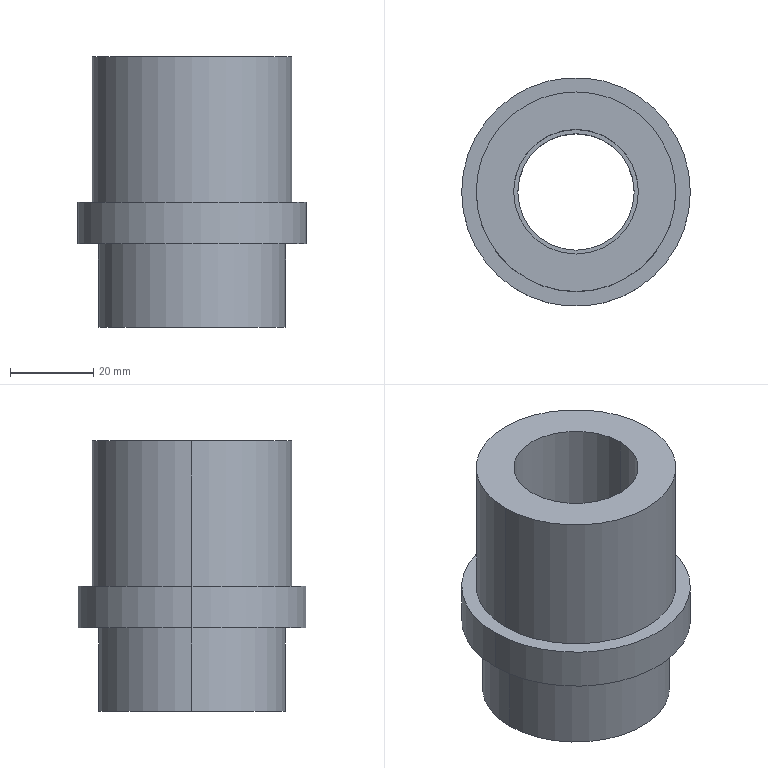Part | SolidWorks | features HoleWzd 1, Revolution 1 | 1 solid | 15 faces | box 55 x 55 x 65 mm | volume 76144 mm3 | cylinder 10 | plane 5 | commonest cylinder face diameters 28 x2 30 x2 45 x2 48 x2 55 x2
STEP:
#1=CARTESIAN_POINT('',(14.,0.,-30.));
#2=VERTEX_POINT('',#1);
#3=CARTESIAN_POINT('',(-14.,0.,-30.));
#4=VERTEX_POINT('',#3);
#5=CARTESIAN_POINT('',(0.,0.,-30.));
#6=DIRECTION('',(0.,0.,-1.));
#7=DIRECTION('',(-1.,0.,0.));
#8=AXIS2_PLACEMENT_3D('',#5,#6,#7);
#9=CIRCLE('',#8,14.);
#10=EDGE_CURVE('',#2,#4,#9,.T.);
#11=ORIENTED_EDGE('',*,*,#10,.F.);
#12=CARTESIAN_POINT('',(14.,0.,-65.));
#13=VERTEX_POINT('',#12);
#14=CARTESIAN_POINT('',(14.,0.,-65.));
#15=DIRECTION('',(0.,0.,-1.));
#16=VECTOR('',#15,1000.);
#17=LINE('',#14,#16);
#18=EDGE_CURVE('',#2,#13,#17,.T.);
#19=ORIENTED_EDGE('',*,*,#18,.T.);
#20=CARTESIAN_POINT('',(-14.,0.,-65.));
#21=VERTEX_POINT('',#20);
#22=CARTESIAN_POINT('',(0.,0.,-65.));
#23=DIRECTION('',(0.,0.,-1.));
#24=DIRECTION('',(-1.,0.,0.));
#25=AXIS2_PLACEMENT_3D('',#22,#23,#24);
#26=CIRCLE('',#25,14.);
#27=EDGE_CURVE('',#13,#21,#26,.T.);
#28=ORIENTED_EDGE('',*,*,#27,.T.);
#29=CARTESIAN_POINT('',(-14.,0.,-65.));
#30=DIRECTION('',(0.,0.,-1.));
#31=VECTOR('',#30,1000.);
#32=LINE('',#29,#31);
#33=EDGE_CURVE('',#4,#21,#32,.T.);
#34=ORIENTED_EDGE('',*,*,#33,.F.);
#35=EDGE_LOOP('',(#11,#19,#28,#34));
#36=FACE_OUTER_BOUND('',#35,.T.);
#37=CARTESIAN_POINT('',(0.,0.,-65.));
#38=DIRECTION('',(0.,0.,-1.));
#39=DIRECTION('',(-1.,0.,0.));
#40=AXIS2_PLACEMENT_3D('',#37,#38,#39);
#41=CYLINDRICAL_SURFACE('',#40,14.);
#42=ADVANCED_FACE('',(#36),#41,.F.);
#43=CARTESIAN_POINT('',(22.5,0.,-65.));
#44=VERTEX_POINT('',#43);
#45=CARTESIAN_POINT('',(-22.5,0.,-65.));
#46=VERTEX_POINT('',#45);
#47=CARTESIAN_POINT('',(0.,0.,-65.));
#48=DIRECTION('',(0.,0.,1.));
#49=DIRECTION('',(1.,0.,0.));
#50=AXIS2_PLACEMENT_3D('',#47,#48,#49);
#51=CIRCLE('',#50,22.5);
#52=EDGE_CURVE('',#44,#46,#51,.T.);
#53=ORIENTED_EDGE('',*,*,#52,.T.);
#54=CARTESIAN_POINT('',(-22.5,0.,-45.));
#55=VERTEX_POINT('',#54);
#56=CARTESIAN_POINT('',(-22.5,0.,0.));
#57=DIRECTION('',(0.,0.,1.));
#58=VECTOR('',#57,1000.);
#59=LINE('',#56,#58);
#60=EDGE_CURVE('',#46,#55,#59,.T.);
#61=ORIENTED_EDGE('',*,*,#60,.T.);
#62=CARTESIAN_POINT('',(22.5,0.,-45.));
#63=VERTEX_POINT('',#62);
#64=CARTESIAN_POINT('',(0.,0.,-45.));
#65=DIRECTION('',(0.,0.,1.));
#66=DIRECTION('',(1.,0.,0.));
#67=AXIS2_PLACEMENT_3D('',#64,#65,#66);
#68=CIRCLE('',#67,22.5);
#69=EDGE_CURVE('',#63,#55,#68,.T.);
#70=ORIENTED_EDGE('',*,*,#69,.F.);
#71=CARTESIAN_POINT('',(22.5,0.,0.));
#72=DIRECTION('',(0.,0.,1.));
#73=VECTOR('',#72,1000.);
#74=LINE('',#71,#73);
#75=EDGE_CURVE('',#44,#63,#74,.T.);
#76=ORIENTED_EDGE('',*,*,#75,.F.);
#77=EDGE_LOOP('',(#53,#61,#70,#76));
#78=FACE_OUTER_BOUND('',#77,.T.);
#79=CARTESIAN_POINT('',(0.,0.,0.));
#80=DIRECTION('',(0.,0.,1.));
#81=DIRECTION('',(1.,0.,0.));
#82=AXIS2_PLACEMENT_3D('',#79,#80,#81);
#83=CYLINDRICAL_SURFACE('',#82,22.5);
#84=ADVANCED_FACE('',(#78),#83,.T.);
#85=CARTESIAN_POINT('',(27.5,0.,-45.));
#86=VERTEX_POINT('',#85);
#87=CARTESIAN_POINT('',(-27.5,0.,-45.));
#88=VERTEX_POINT('',#87);
#89=CARTESIAN_POINT('',(0.,0.,-45.));
#90=DIRECTION('',(0.,0.,1.));
#91=DIRECTION('',(1.,0.,0.));
#92=AXIS2_PLACEMENT_3D('',#89,#90,#91);
#93=CIRCLE('',#92,27.5);
#94=EDGE_CURVE('',#86,#88,#93,.T.);
#95=ORIENTED_EDGE('',*,*,#94,.T.);
#96=CARTESIAN_POINT('',(-27.5,0.,-35.));
#97=VERTEX_POINT('',#96);
#98=CARTESIAN_POINT('',(-27.5,0.,0.));
#99=DIRECTION('',(0.,0.,1.));
#100=VECTOR('',#99,1000.);
#101=LINE('',#98,#100);
#102=EDGE_CURVE('',#88,#97,#101,.T.);
#103=ORIENTED_EDGE('',*,*,#102,.T.);
#104=CARTESIAN_POINT('',(27.5,0.,-35.));
#105=VERTEX_POINT('',#104);
#106=CARTESIAN_POINT('',(0.,0.,-35.));
#107=DIRECTION('',(0.,0.,1.));
#108=DIRECTION('',(1.,0.,0.));
#109=AXIS2_PLACEMENT_3D('',#106,#107,#108);
#110=CIRCLE('',#109,27.5);
#111=EDGE_CURVE('',#105,#97,#110,.T.);
#112=ORIENTED_EDGE('',*,*,#111,.F.);
#113=CARTESIAN_POINT('',(27.5,0.,0.));
#114=DIRECTION('',(0.,0.,1.));
#115=VECTOR('',#114,1000.);
#116=LINE('',#113,#115);
#117=EDGE_CURVE('',#86,#105,#116,.T.);
#118=ORIENTED_EDGE('',*,*,#117,.F.);
#119=EDGE_LOOP('',(#95,#103,#112,#118));
#120=FACE_OUTER_BOUND('',#119,.T.);
#121=CARTESIAN_POINT('',(0.,0.,0.));
#122=DIRECTION('',(0.,0.,1.));
#123=DIRECTION('',(1.,0.,0.));
#124=AXIS2_PLACEMENT_3D('',#121,#122,#123);
#125=CYLINDRICAL_SURFACE('',#124,27.5);
#126=ADVANCED_FACE('',(#120),#125,.T.);
#127=CARTESIAN_POINT('',(24.,0.,-35.));
#128=VERTEX_POINT('',#127);
#129=CARTESIAN_POINT('',(-24.,0.,-35.));
#130=VERTEX_POINT('',#129);
#131=CARTESIAN_POINT('',(0.,0.,-35.));
#132=DIRECTION('',(0.,0.,1.));
#133=DIRECTION('',(1.,0.,0.));
#134=AXIS2_PLACEMENT_3D('',#131,#132,#133);
#135=CIRCLE('',#134,24.);
#136=EDGE_CURVE('',#128,#130,#135,.T.);
#137=ORIENTED_EDGE('',*,*,#136,.T.);
#138=CARTESIAN_POINT('',(-24.,0.,0.));
#139=VERTEX_POINT('',#138);
#140=CARTESIAN_POINT('',(-24.,0.,0.));
#141=DIRECTION('',(0.,0.,1.));
#142=VECTOR('',#141,1000.);
#143=LINE('',#140,#142);
#144=EDGE_CURVE('',#130,#139,#143,.T.);
#145=ORIENTED_EDGE('',*,*,#144,.T.);
#146=CARTESIAN_POINT('',(24.,0.,0.));
#147=VERTEX_POINT('',#146);
#148=CARTESIAN_POINT('',(0.,0.,0.));
#149=DIRECTION('',(0.,0.,1.));
#150=DIRECTION('',(1.,0.,0.));
#151=AXIS2_PLACEMENT_3D('',#148,#149,#150);
#152=CIRCLE('',#151,24.);
#153=EDGE_CURVE('',#147,#139,#152,.T.);
#154=ORIENTED_EDGE('',*,*,#153,.F.);
#155=CARTESIAN_POINT('',(24.,0.,0.));
#156=DIRECTION('',(0.,0.,1.));
#157=VECTOR('',#156,1000.);
#158=LINE('',#155,#157);
#159=EDGE_CURVE('',#128,#147,#158,.T.);
#160=ORIENTED_EDGE('',*,*,#159,.F.);
#161=EDGE_LOOP('',(#137,#145,#154,#160));
#162=FACE_OUTER_BOUND('',#161,.T.);
#163=CARTESIAN_POINT('',(0.,0.,0.));
#164=DIRECTION('',(0.,0.,1.));
#165=DIRECTION('',(1.,0.,0.));
#166=AXIS2_PLACEMENT_3D('',#163,#164,#165);
#167=CYLINDRICAL_SURFACE('',#166,24.);
#168=ADVANCED_FACE('',(#162),#167,.T.);
#169=CARTESIAN_POINT('',(-15.,0.,-30.));
#170=VERTEX_POINT('',#169);
#171=CARTESIAN_POINT('',(15.,0.,-30.));
#172=VERTEX_POINT('',#171);
#173=CARTESIAN_POINT('',(0.,0.,-30.));
#174=DIRECTION('',(0.,0.,1.));
#175=DIRECTION('',(1.,0.,0.));
#176=AXIS2_PLACEMENT_3D('',#173,#174,#175);
#177=CIRCLE('',#176,15.);
#178=EDGE_CURVE('',#170,#172,#177,.T.);
#179=ORIENTED_EDGE('',*,*,#178,.F.);
#180=CARTESIAN_POINT('',(-15.,0.,0.));
#181=VERTEX_POINT('',#180);
#182=CARTESIAN_POINT('',(-15.,0.,0.));
#183=DIRECTION('',(0.,0.,1.));
#184=VECTOR('',#183,1000.);
#185=LINE('',#182,#184);
#186=EDGE_CURVE('',#170,#181,#185,.T.);
#187=ORIENTED_EDGE('',*,*,#186,.T.);
#188=CARTESIAN_POINT('',(15.,0.,0.));
#189=VERTEX_POINT('',#188);
#190=CARTESIAN_POINT('',(0.,0.,0.));
#191=DIRECTION('',(0.,0.,1.));
#192=DIRECTION('',(1.,0.,0.));
#193=AXIS2_PLACEMENT_3D('',#190,#191,#192);
#194=CIRCLE('',#193,15.);
#195=EDGE_CURVE('',#181,#189,#194,.T.);
#196=ORIENTED_EDGE('',*,*,#195,.T.);
#197=CARTESIAN_POINT('',(15.,0.,0.));
#198=DIRECTION('',(0.,0.,1.));
#199=VECTOR('',#198,1000.);
#200=LINE('',#197,#199);
#201=EDGE_CURVE('',#172,#189,#200,.T.);
#202=ORIENTED_EDGE('',*,*,#201,.F.);
#203=EDGE_LOOP('',(#179,#187,#196,#202));
#204=FACE_OUTER_BOUND('',#203,.T.);
#205=CARTESIAN_POINT('',(0.,0.,0.));
#206=DIRECTION('',(0.,0.,1.));
#207=DIRECTION('',(1.,0.,0.));
#208=AXIS2_PLACEMENT_3D('',#205,#206,#207);
#209=CYLINDRICAL_SURFACE('',#208,15.);
#210=ADVANCED_FACE('',(#204),#209,.F.);
#211=ORIENTED_EDGE('',*,*,#186,.F.);
#212=CARTESIAN_POINT('',(0.,0.,-30.));
#213=DIRECTION('',(0.,0.,1.));
#214=DIRECTION('',(1.,0.,0.));
#215=AXIS2_PLACEMENT_3D('',#212,#213,#214);
#216=CIRCLE('',#215,15.);
#217=EDGE_CURVE('',#172,#170,#216,.T.);
#218=ORIENTED_EDGE('',*,*,#217,.F.);
#219=ORIENTED_EDGE('',*,*,#201,.T.);
#220=CARTESIAN_POINT('',(0.,0.,0.));
#221=DIRECTION('',(0.,0.,1.));
#222=DIRECTION('',(1.,0.,0.));
#223=AXIS2_PLACEMENT_3D('',#220,#221,#222);
#224=CIRCLE('',#223,15.);
#225=EDGE_CURVE('',#189,#181,#224,.T.);
#226=ORIENTED_EDGE('',*,*,#225,.T.);
#227=EDGE_LOOP('',(#211,#218,#219,#226));
#228=FACE_OUTER_BOUND('',#227,.T.);
#229=CARTESIAN_POINT('',(0.,0.,0.));
#230=DIRECTION('',(0.,0.,1.));
#231=DIRECTION('',(1.,0.,0.));
#232=AXIS2_PLACEMENT_3D('',#229,#230,#231);
#233=CYLINDRICAL_SURFACE('',#232,15.);
#234=ADVANCED_FACE('',(#228),#233,.F.);
#235=ORIENTED_EDGE('',*,*,#153,.T.);
#236=CARTESIAN_POINT('',(0.,0.,0.));
#237=DIRECTION('',(0.,0.,1.));
#238=DIRECTION('',(1.,0.,0.));
#239=AXIS2_PLACEMENT_3D('',#236,#237,#238);
#240=CIRCLE('',#239,24.);
#241=EDGE_CURVE('',#139,#147,#240,.T.);
#242=ORIENTED_EDGE('',*,*,#241,.T.);
#243=EDGE_LOOP('',(#235,#242));
#244=FACE_OUTER_BOUND('',#243,.T.);
#245=ORIENTED_EDGE('',*,*,#225,.F.);
#246=ORIENTED_EDGE('',*,*,#195,.F.);
#247=EDGE_LOOP('',(#245,#246));
#248=FACE_BOUND('',#247,.T.);
#249=CARTESIAN_POINT('',(15.,0.,0.));
#250=DIRECTION('',(0.,0.,1.));
#251=DIRECTION('',(1.,0.,0.));
#252=AXIS2_PLACEMENT_3D('',#249,#250,#251);
#253=PLANE('',#252);
#254=ADVANCED_FACE('',(#244,#248),#253,.T.);
#255=ORIENTED_EDGE('',*,*,#144,.F.);
#256=CARTESIAN_POINT('',(0.,0.,-35.));
#257=DIRECTION('',(0.,0.,1.));
#258=DIRECTION('',(1.,0.,0.));
#259=AXIS2_PLACEMENT_3D('',#256,#257,#258);
#260=CIRCLE('',#259,24.);
#261=EDGE_CURVE('',#130,#128,#260,.T.);
#262=ORIENTED_EDGE('',*,*,#261,.T.);
#263=ORIENTED_EDGE('',*,*,#159,.T.);
#264=ORIENTED_EDGE('',*,*,#241,.F.);
#265=EDGE_LOOP('',(#255,#262,#263,#264));
#266=FACE_OUTER_BOUND('',#265,.T.);
#267=CARTESIAN_POINT('',(0.,0.,0.));
#268=DIRECTION('',(0.,0.,1.));
#269=DIRECTION('',(1.,0.,0.));
#270=AXIS2_PLACEMENT_3D('',#267,#268,#269);
#271=CYLINDRICAL_SURFACE('',#270,24.);
#272=ADVANCED_FACE('',(#266),#271,.T.);
#273=ORIENTED_EDGE('',*,*,#111,.T.);
#274=CARTESIAN_POINT('',(0.,0.,-35.));
#275=DIRECTION('',(0.,0.,1.));
#276=DIRECTION('',(1.,0.,0.));
#277=AXIS2_PLACEMENT_3D('',#274,#275,#276);
#278=CIRCLE('',#277,27.5);
#279=EDGE_CURVE('',#97,#105,#278,.T.);
#280=ORIENTED_EDGE('',*,*,#279,.T.);
#281=EDGE_LOOP('',(#273,#280));
#282=FACE_OUTER_BOUND('',#281,.T.);
#283=ORIENTED_EDGE('',*,*,#136,.F.);
#284=ORIENTED_EDGE('',*,*,#261,.F.);
#285=EDGE_LOOP('',(#283,#284));
#286=FACE_BOUND('',#285,.T.);
#287=CARTESIAN_POINT('',(24.,0.,-35.));
#288=DIRECTION('',(0.,0.,1.));
#289=DIRECTION('',(1.,0.,0.));
#290=AXIS2_PLACEMENT_3D('',#287,#288,#289);
#291=PLANE('',#290);
#292=ADVANCED_FACE('',(#282,#286),#291,.T.);
#293=ORIENTED_EDGE('',*,*,#102,.F.);
#294=CARTESIAN_POINT('',(0.,0.,-45.));
#295=DIRECTION('',(0.,0.,1.));
#296=DIRECTION('',(1.,0.,0.));
#297=AXIS2_PLACEMENT_3D('',#294,#295,#296);
#298=CIRCLE('',#297,27.5);
#299=EDGE_CURVE('',#88,#86,#298,.T.);
#300=ORIENTED_EDGE('',*,*,#299,.T.);
#301=ORIENTED_EDGE('',*,*,#117,.T.);
#302=ORIENTED_EDGE('',*,*,#279,.F.);
#303=EDGE_LOOP('',(#293,#300,#301,#302));
#304=FACE_OUTER_BOUND('',#303,.T.);
#305=CARTESIAN_POINT('',(0.,0.,0.));
#306=DIRECTION('',(0.,0.,1.));
#307=DIRECTION('',(1.,0.,0.));
#308=AXIS2_PLACEMENT_3D('',#305,#306,#307);
#309=CYLINDRICAL_SURFACE('',#308,27.5);
#310=ADVANCED_FACE('',(#304),#309,.T.);
#311=ORIENTED_EDGE('',*,*,#69,.T.);
#312=CARTESIAN_POINT('',(0.,0.,-45.));
#313=DIRECTION('',(0.,0.,1.));
#314=DIRECTION('',(1.,0.,0.));
#315=AXIS2_PLACEMENT_3D('',#312,#313,#314);
#316=CIRCLE('',#315,22.5);
#317=EDGE_CURVE('',#55,#63,#316,.T.);
#318=ORIENTED_EDGE('',*,*,#317,.T.);
#319=EDGE_LOOP('',(#311,#318));
#320=FACE_BOUND('',#319,.T.);
#321=ORIENTED_EDGE('',*,*,#94,.F.);
#322=ORIENTED_EDGE('',*,*,#299,.F.);
#323=EDGE_LOOP('',(#321,#322));
#324=FACE_OUTER_BOUND('',#323,.T.);
#325=CARTESIAN_POINT('',(27.5,0.,-45.));
#326=DIRECTION('',(0.,0.,-1.));
#327=DIRECTION('',(-1.,0.,0.));
#328=AXIS2_PLACEMENT_3D('',#325,#326,#327);
#329=PLANE('',#328);
#330=ADVANCED_FACE('',(#320,#324),#329,.T.);
#331=ORIENTED_EDGE('',*,*,#60,.F.);
#332=CARTESIAN_POINT('',(0.,0.,-65.));
#333=DIRECTION('',(0.,0.,1.));
#334=DIRECTION('',(1.,0.,0.));
#335=AXIS2_PLACEMENT_3D('',#332,#333,#334);
#336=CIRCLE('',#335,22.5);
#337=EDGE_CURVE('',#46,#44,#336,.T.);
#338=ORIENTED_EDGE('',*,*,#337,.T.);
#339=ORIENTED_EDGE('',*,*,#75,.T.);
#340=ORIENTED_EDGE('',*,*,#317,.F.);
#341=EDGE_LOOP('',(#331,#338,#339,#340));
#342=FACE_OUTER_BOUND('',#341,.T.);
#343=CARTESIAN_POINT('',(0.,0.,0.));
#344=DIRECTION('',(0.,0.,1.));
#345=DIRECTION('',(1.,0.,0.));
#346=AXIS2_PLACEMENT_3D('',#343,#344,#345);
#347=CYLINDRICAL_SURFACE('',#346,22.5);
#348=ADVANCED_FACE('',(#342),#347,.T.);
#349=CARTESIAN_POINT('',(0.,0.,-65.));
#350=DIRECTION('',(0.,0.,-1.));
#351=DIRECTION('',(-1.,0.,0.));
#352=AXIS2_PLACEMENT_3D('',#349,#350,#351);
#353=CIRCLE('',#352,14.);
#354=EDGE_CURVE('',#21,#13,#353,.T.);
#355=ORIENTED_EDGE('',*,*,#354,.F.);
#356=ORIENTED_EDGE('',*,*,#27,.F.);
#357=EDGE_LOOP('',(#355,#356));
#358=FACE_BOUND('',#357,.T.);
#359=ORIENTED_EDGE('',*,*,#52,.F.);
#360=ORIENTED_EDGE('',*,*,#337,.F.);
#361=EDGE_LOOP('',(#359,#360));
#362=FACE_OUTER_BOUND('',#361,.T.);
#363=CARTESIAN_POINT('',(22.5,0.,-65.));
#364=DIRECTION('',(0.,0.,-1.));
#365=DIRECTION('',(-1.,0.,0.));
#366=AXIS2_PLACEMENT_3D('',#363,#364,#365);
#367=PLANE('',#366);
#368=ADVANCED_FACE('',(#358,#362),#367,.T.);
#369=CARTESIAN_POINT('',(0.,0.,-30.));
#370=DIRECTION('',(0.,0.,-1.));
#371=DIRECTION('',(-1.,0.,0.));
#372=AXIS2_PLACEMENT_3D('',#369,#370,#371);
#373=CIRCLE('',#372,14.);
#374=EDGE_CURVE('',#4,#2,#373,.T.);
#375=ORIENTED_EDGE('',*,*,#374,.T.);
#376=ORIENTED_EDGE('',*,*,#10,.T.);
#377=EDGE_LOOP('',(#375,#376));
#378=FACE_BOUND('',#377,.T.);
#379=ORIENTED_EDGE('',*,*,#217,.T.);
#380=ORIENTED_EDGE('',*,*,#178,.T.);
#381=EDGE_LOOP('',(#379,#380));
#382=FACE_OUTER_BOUND('',#381,.T.);
#383=CARTESIAN_POINT('',(12.5,0.,-30.));
#384=DIRECTION('',(0.,0.,1.));
#385=DIRECTION('',(1.,0.,0.));
#386=AXIS2_PLACEMENT_3D('',#383,#384,#385);
#387=PLANE('',#386);
#388=ADVANCED_FACE('',(#378,#382),#387,.T.);
#389=ORIENTED_EDGE('',*,*,#18,.F.);
#390=ORIENTED_EDGE('',*,*,#374,.F.);
#391=ORIENTED_EDGE('',*,*,#33,.T.);
#392=ORIENTED_EDGE('',*,*,#354,.T.);
#393=EDGE_LOOP('',(#389,#390,#391,#392));
#394=FACE_OUTER_BOUND('',#393,.T.);
#395=CARTESIAN_POINT('',(0.,0.,-65.));
#396=DIRECTION('',(0.,0.,-1.));
#397=DIRECTION('',(-1.,0.,0.));
#398=AXIS2_PLACEMENT_3D('',#395,#396,#397);
#399=CYLINDRICAL_SURFACE('',#398,14.);
#400=ADVANCED_FACE('',(#394),#399,.F.);
#401=CLOSED_SHELL('',(#42,#84,#126,#168,#210,#234,#254,#272,#292,#310,#330,#348,#368,#388,#400));
#402=MANIFOLD_SOLID_BREP('',#401);
#403=CARTESIAN_POINT('',(0.,0.,0.));
#404=DIRECTION('',(0.,0.,1.));
#405=DIRECTION('',(1.,0.,0.));
#406=AXIS2_PLACEMENT_3D('',#403,#404,#405);
#407=(LENGTH_UNIT()NAMED_UNIT(*)SI_UNIT(.MILLI.,.METRE.));
#408=UNCERTAINTY_MEASURE_WITH_UNIT(LENGTH_MEASURE(0.00001),#407,'','');
#409=(NAMED_UNIT(*)PLANE_ANGLE_UNIT()SI_UNIT($,.RADIAN.));
#410=(NAMED_UNIT(*)SI_UNIT($,.STERADIAN.)SOLID_ANGLE_UNIT());
#411=(GEOMETRIC_REPRESENTATION_CONTEXT(3)GLOBAL_UNCERTAINTY_ASSIGNED_CONTEXT((#408))GLOBAL_UNIT_ASSIGNED_CONTEXT((#407,#409,#410))REPRESENTATION_CONTEXT('',''));
#412=ADVANCED_BREP_SHAPE_REPRESENTATION('',(#402,#406),#411);